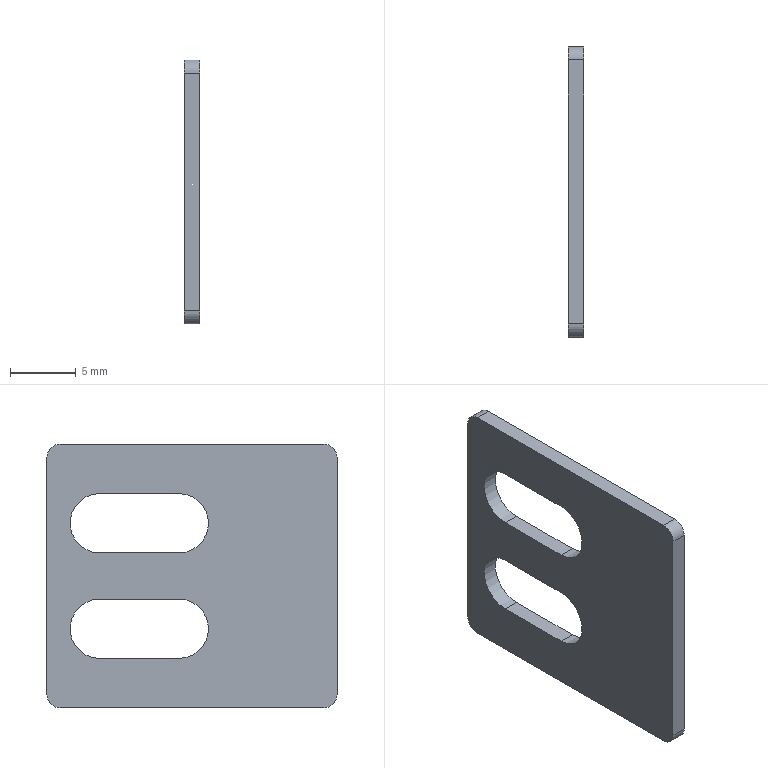Part | SolidWorks | features Fillet 1, FlatPattern 1, HoleWzd 1, SMBaseFlange 1, SheetMetal 1 | 1 solid | 18 faces | box 1.2 x 22 x 20 mm | volume 424 mm3 | plane 10 | cylinder 8 | commonest cylinder face diameters 2 x4 4.5 x4
STEP:
#1=CARTESIAN_POINT('',(-1.2,-10.,-10.));
#2=VERTEX_POINT('',#1);
#3=CARTESIAN_POINT('',(-1.2,10.,-10.));
#4=VERTEX_POINT('',#3);
#5=CARTESIAN_POINT('',(-1.2,-11.,-10.));
#6=DIRECTION('',(0.,1.,0.));
#7=VECTOR('',#6,1000.);
#8=LINE('',#5,#7);
#9=EDGE_CURVE('',#2,#4,#8,.T.);
#10=ORIENTED_EDGE('',*,*,#9,.T.);
#11=CARTESIAN_POINT('',(0.,10.,-10.));
#12=VERTEX_POINT('',#11);
#13=CARTESIAN_POINT('',(-1.2,10.,-10.));
#14=DIRECTION('',(1.,0.,0.));
#15=VECTOR('',#14,1000.);
#16=LINE('',#13,#15);
#17=EDGE_CURVE('',#4,#12,#16,.T.);
#18=ORIENTED_EDGE('',*,*,#17,.T.);
#19=CARTESIAN_POINT('',(0.,-10.,-10.));
#20=VERTEX_POINT('',#19);
#21=CARTESIAN_POINT('',(0.,-11.,-10.));
#22=DIRECTION('',(0.,1.,0.));
#23=VECTOR('',#22,1000.);
#24=LINE('',#21,#23);
#25=EDGE_CURVE('',#20,#12,#24,.T.);
#26=ORIENTED_EDGE('',*,*,#25,.F.);
#27=CARTESIAN_POINT('',(-1.2,-10.,-10.));
#28=DIRECTION('',(-1.,0.,0.));
#29=VECTOR('',#28,1000.);
#30=LINE('',#27,#29);
#31=EDGE_CURVE('',#20,#2,#30,.T.);
#32=ORIENTED_EDGE('',*,*,#31,.T.);
#33=EDGE_LOOP('',(#10,#18,#26,#32));
#34=FACE_OUTER_BOUND('',#33,.T.);
#35=CARTESIAN_POINT('',(-1.2,-11.,-10.));
#36=DIRECTION('',(0.,0.,-1.));
#37=DIRECTION('',(-1.,0.,0.));
#38=AXIS2_PLACEMENT_3D('',#35,#36,#37);
#39=PLANE('',#38);
#40=ADVANCED_FACE('',(#34),#39,.T.);
#41=CARTESIAN_POINT('',(0.,-11.,9.));
#42=VERTEX_POINT('',#41);
#43=CARTESIAN_POINT('',(0.,-11.,-9.));
#44=VERTEX_POINT('',#43);
#45=CARTESIAN_POINT('',(0.,-11.,10.));
#46=DIRECTION('',(0.,0.,-1.));
#47=VECTOR('',#46,1000.);
#48=LINE('',#45,#47);
#49=EDGE_CURVE('',#42,#44,#48,.T.);
#50=ORIENTED_EDGE('',*,*,#49,.F.);
#51=CARTESIAN_POINT('',(-1.2,-11.,9.));
#52=VERTEX_POINT('',#51);
#53=CARTESIAN_POINT('',(-1.2,-11.,9.));
#54=DIRECTION('',(-1.,0.,0.));
#55=VECTOR('',#54,1000.);
#56=LINE('',#53,#55);
#57=EDGE_CURVE('',#42,#52,#56,.T.);
#58=ORIENTED_EDGE('',*,*,#57,.T.);
#59=CARTESIAN_POINT('',(-1.2,-11.,-9.));
#60=VERTEX_POINT('',#59);
#61=CARTESIAN_POINT('',(-1.2,-11.,10.));
#62=DIRECTION('',(0.,0.,-1.));
#63=VECTOR('',#62,1000.);
#64=LINE('',#61,#63);
#65=EDGE_CURVE('',#52,#60,#64,.T.);
#66=ORIENTED_EDGE('',*,*,#65,.T.);
#67=CARTESIAN_POINT('',(-1.2,-11.,-9.));
#68=DIRECTION('',(1.,0.,0.));
#69=VECTOR('',#68,1000.);
#70=LINE('',#67,#69);
#71=EDGE_CURVE('',#60,#44,#70,.T.);
#72=ORIENTED_EDGE('',*,*,#71,.T.);
#73=EDGE_LOOP('',(#50,#58,#66,#72));
#74=FACE_OUTER_BOUND('',#73,.T.);
#75=CARTESIAN_POINT('',(-1.2,-11.,10.));
#76=DIRECTION('',(0.,-1.,0.));
#77=DIRECTION('',(0.,0.,-1.));
#78=AXIS2_PLACEMENT_3D('',#75,#76,#77);
#79=PLANE('',#78);
#80=ADVANCED_FACE('',(#74),#79,.T.);
#81=CARTESIAN_POINT('',(0.,10.,10.));
#82=VERTEX_POINT('',#81);
#83=CARTESIAN_POINT('',(0.,-10.,10.));
#84=VERTEX_POINT('',#83);
#85=CARTESIAN_POINT('',(0.,-11.,10.));
#86=DIRECTION('',(0.,-1.,0.));
#87=VECTOR('',#86,1000.);
#88=LINE('',#85,#87);
#89=EDGE_CURVE('',#82,#84,#88,.T.);
#90=ORIENTED_EDGE('',*,*,#89,.F.);
#91=CARTESIAN_POINT('',(-1.2,10.,10.));
#92=VERTEX_POINT('',#91);
#93=CARTESIAN_POINT('',(-1.2,10.,10.));
#94=DIRECTION('',(-1.,0.,0.));
#95=VECTOR('',#94,1000.);
#96=LINE('',#93,#95);
#97=EDGE_CURVE('',#82,#92,#96,.T.);
#98=ORIENTED_EDGE('',*,*,#97,.T.);
#99=CARTESIAN_POINT('',(-1.2,-10.,10.));
#100=VERTEX_POINT('',#99);
#101=CARTESIAN_POINT('',(-1.2,-11.,10.));
#102=DIRECTION('',(0.,-1.,0.));
#103=VECTOR('',#102,1000.);
#104=LINE('',#101,#103);
#105=EDGE_CURVE('',#92,#100,#104,.T.);
#106=ORIENTED_EDGE('',*,*,#105,.T.);
#107=CARTESIAN_POINT('',(-1.2,-10.,10.));
#108=DIRECTION('',(1.,0.,0.));
#109=VECTOR('',#108,1000.);
#110=LINE('',#107,#109);
#111=EDGE_CURVE('',#100,#84,#110,.T.);
#112=ORIENTED_EDGE('',*,*,#111,.T.);
#113=EDGE_LOOP('',(#90,#98,#106,#112));
#114=FACE_OUTER_BOUND('',#113,.T.);
#115=CARTESIAN_POINT('',(-1.2,-11.,10.));
#116=DIRECTION('',(0.,0.,1.));
#117=DIRECTION('',(1.,0.,0.));
#118=AXIS2_PLACEMENT_3D('',#115,#116,#117);
#119=PLANE('',#118);
#120=ADVANCED_FACE('',(#114),#119,.T.);
#121=CARTESIAN_POINT('',(-1.2,11.,-9.));
#122=VERTEX_POINT('',#121);
#123=CARTESIAN_POINT('',(-1.2,11.,9.));
#124=VERTEX_POINT('',#123);
#125=CARTESIAN_POINT('',(-1.2,11.,10.));
#126=DIRECTION('',(0.,0.,1.));
#127=VECTOR('',#126,1000.);
#128=LINE('',#125,#127);
#129=EDGE_CURVE('',#122,#124,#128,.T.);
#130=ORIENTED_EDGE('',*,*,#129,.T.);
#131=CARTESIAN_POINT('',(0.,11.,9.));
#132=VERTEX_POINT('',#131);
#133=CARTESIAN_POINT('',(-1.2,11.,9.));
#134=DIRECTION('',(1.,0.,0.));
#135=VECTOR('',#134,1000.);
#136=LINE('',#133,#135);
#137=EDGE_CURVE('',#124,#132,#136,.T.);
#138=ORIENTED_EDGE('',*,*,#137,.T.);
#139=CARTESIAN_POINT('',(0.,11.,-9.));
#140=VERTEX_POINT('',#139);
#141=CARTESIAN_POINT('',(0.,11.,10.));
#142=DIRECTION('',(0.,0.,1.));
#143=VECTOR('',#142,1000.);
#144=LINE('',#141,#143);
#145=EDGE_CURVE('',#140,#132,#144,.T.);
#146=ORIENTED_EDGE('',*,*,#145,.F.);
#147=CARTESIAN_POINT('',(-1.2,11.,-9.));
#148=DIRECTION('',(-1.,0.,0.));
#149=VECTOR('',#148,1000.);
#150=LINE('',#147,#149);
#151=EDGE_CURVE('',#140,#122,#150,.T.);
#152=ORIENTED_EDGE('',*,*,#151,.T.);
#153=EDGE_LOOP('',(#130,#138,#146,#152));
#154=FACE_OUTER_BOUND('',#153,.T.);
#155=CARTESIAN_POINT('',(-1.2,11.,10.));
#156=DIRECTION('',(0.,1.,0.));
#157=DIRECTION('',(0.,0.,1.));
#158=AXIS2_PLACEMENT_3D('',#155,#156,#157);
#159=PLANE('',#158);
#160=ADVANCED_FACE('',(#154),#159,.T.);
#161=CARTESIAN_POINT('',(-1.2,1.,-1.75));
#162=VERTEX_POINT('',#161);
#163=CARTESIAN_POINT('',(-1.2,7.,-1.75));
#164=VERTEX_POINT('',#163);
#165=CARTESIAN_POINT('',(-1.2,1.,-1.75));
#166=DIRECTION('',(0.,1.,0.));
#167=VECTOR('',#166,1000.);
#168=LINE('',#165,#167);
#169=EDGE_CURVE('',#162,#164,#168,.T.);
#170=ORIENTED_EDGE('',*,*,#169,.F.);
#171=CARTESIAN_POINT('',(-1.2,1.,-6.25));
#172=VERTEX_POINT('',#171);
#173=CARTESIAN_POINT('',(-1.2,1.,-4.));
#174=DIRECTION('',(-1.,0.,0.));
#175=DIRECTION('',(0.,0.,1.));
#176=AXIS2_PLACEMENT_3D('',#173,#174,#175);
#177=CIRCLE('',#176,2.25);
#178=EDGE_CURVE('',#172,#162,#177,.T.);
#179=ORIENTED_EDGE('',*,*,#178,.F.);
#180=CARTESIAN_POINT('',(-1.2,7.,-6.25));
#181=VERTEX_POINT('',#180);
#182=CARTESIAN_POINT('',(-1.2,1.,-6.25));
#183=DIRECTION('',(0.,1.,0.));
#184=VECTOR('',#183,1000.);
#185=LINE('',#182,#184);
#186=EDGE_CURVE('',#172,#181,#185,.T.);
#187=ORIENTED_EDGE('',*,*,#186,.T.);
#188=CARTESIAN_POINT('',(-1.2,7.,-4.));
#189=DIRECTION('',(-1.,0.,0.));
#190=DIRECTION('',(0.,0.,1.));
#191=AXIS2_PLACEMENT_3D('',#188,#189,#190);
#192=CIRCLE('',#191,2.25);
#193=EDGE_CURVE('',#164,#181,#192,.T.);
#194=ORIENTED_EDGE('',*,*,#193,.F.);
#195=EDGE_LOOP('',(#170,#179,#187,#194));
#196=FACE_BOUND('',#195,.T.);
#197=CARTESIAN_POINT('',(-1.2,1.,1.75));
#198=VERTEX_POINT('',#197);
#199=CARTESIAN_POINT('',(-1.2,1.,6.25));
#200=VERTEX_POINT('',#199);
#201=CARTESIAN_POINT('',(-1.2,1.,4.));
#202=DIRECTION('',(-1.,0.,0.));
#203=DIRECTION('',(0.,0.,1.));
#204=AXIS2_PLACEMENT_3D('',#201,#202,#203);
#205=CIRCLE('',#204,2.25);
#206=EDGE_CURVE('',#198,#200,#205,.T.);
#207=ORIENTED_EDGE('',*,*,#206,.F.);
#208=CARTESIAN_POINT('',(-1.2,7.,1.75));
#209=VERTEX_POINT('',#208);
#210=CARTESIAN_POINT('',(-1.2,1.,1.75));
#211=DIRECTION('',(0.,1.,0.));
#212=VECTOR('',#211,1000.);
#213=LINE('',#210,#212);
#214=EDGE_CURVE('',#198,#209,#213,.T.);
#215=ORIENTED_EDGE('',*,*,#214,.T.);
#216=CARTESIAN_POINT('',(-1.2,7.,6.25));
#217=VERTEX_POINT('',#216);
#218=CARTESIAN_POINT('',(-1.2,7.,4.));
#219=DIRECTION('',(-1.,0.,0.));
#220=DIRECTION('',(0.,0.,1.));
#221=AXIS2_PLACEMENT_3D('',#218,#219,#220);
#222=CIRCLE('',#221,2.25);
#223=EDGE_CURVE('',#217,#209,#222,.T.);
#224=ORIENTED_EDGE('',*,*,#223,.F.);
#225=CARTESIAN_POINT('',(-1.2,1.,6.25));
#226=DIRECTION('',(0.,1.,0.));
#227=VECTOR('',#226,1000.);
#228=LINE('',#225,#227);
#229=EDGE_CURVE('',#200,#217,#228,.T.);
#230=ORIENTED_EDGE('',*,*,#229,.F.);
#231=EDGE_LOOP('',(#207,#215,#224,#230));
#232=FACE_BOUND('',#231,.T.);
#233=ORIENTED_EDGE('',*,*,#105,.F.);
#234=CARTESIAN_POINT('',(-1.2,10.,9.));
#235=DIRECTION('',(-1.,0.,0.));
#236=DIRECTION('',(0.,0.,1.));
#237=AXIS2_PLACEMENT_3D('',#234,#235,#236);
#238=CIRCLE('',#237,1.);
#239=EDGE_CURVE('',#92,#124,#238,.T.);
#240=ORIENTED_EDGE('',*,*,#239,.T.);
#241=ORIENTED_EDGE('',*,*,#129,.F.);
#242=CARTESIAN_POINT('',(-1.2,10.,-9.));
#243=DIRECTION('',(-1.,0.,0.));
#244=DIRECTION('',(0.,0.,1.));
#245=AXIS2_PLACEMENT_3D('',#242,#243,#244);
#246=CIRCLE('',#245,1.);
#247=EDGE_CURVE('',#122,#4,#246,.T.);
#248=ORIENTED_EDGE('',*,*,#247,.T.);
#249=ORIENTED_EDGE('',*,*,#9,.F.);
#250=CARTESIAN_POINT('',(-1.2,-10.,-9.));
#251=DIRECTION('',(-1.,0.,0.));
#252=DIRECTION('',(0.,0.,1.));
#253=AXIS2_PLACEMENT_3D('',#250,#251,#252);
#254=CIRCLE('',#253,1.);
#255=EDGE_CURVE('',#2,#60,#254,.T.);
#256=ORIENTED_EDGE('',*,*,#255,.T.);
#257=ORIENTED_EDGE('',*,*,#65,.F.);
#258=CARTESIAN_POINT('',(-1.2,-10.,9.));
#259=DIRECTION('',(-1.,0.,0.));
#260=DIRECTION('',(0.,0.,1.));
#261=AXIS2_PLACEMENT_3D('',#258,#259,#260);
#262=CIRCLE('',#261,1.);
#263=EDGE_CURVE('',#52,#100,#262,.T.);
#264=ORIENTED_EDGE('',*,*,#263,.T.);
#265=EDGE_LOOP('',(#233,#240,#241,#248,#249,#256,#257,#264));
#266=FACE_OUTER_BOUND('',#265,.T.);
#267=CARTESIAN_POINT('',(-1.2,0.,0.));
#268=DIRECTION('',(-1.,0.,0.));
#269=DIRECTION('',(0.,0.,1.));
#270=AXIS2_PLACEMENT_3D('',#267,#268,#269);
#271=PLANE('',#270);
#272=ADVANCED_FACE('',(#196,#232,#266),#271,.T.);
#273=CARTESIAN_POINT('',(0.,1.,-6.25));
#274=VERTEX_POINT('',#273);
#275=CARTESIAN_POINT('',(0.,1.,-1.75));
#276=VERTEX_POINT('',#275);
#277=CARTESIAN_POINT('',(0.,1.,-4.));
#278=DIRECTION('',(-1.,0.,0.));
#279=DIRECTION('',(0.,0.,1.));
#280=AXIS2_PLACEMENT_3D('',#277,#278,#279);
#281=CIRCLE('',#280,2.25);
#282=EDGE_CURVE('',#274,#276,#281,.T.);
#283=ORIENTED_EDGE('',*,*,#282,.T.);
#284=CARTESIAN_POINT('',(0.,7.,-1.75));
#285=VERTEX_POINT('',#284);
#286=CARTESIAN_POINT('',(0.,0.,-1.75));
#287=DIRECTION('',(0.,1.,0.));
#288=VECTOR('',#287,1000.);
#289=LINE('',#286,#288);
#290=EDGE_CURVE('',#276,#285,#289,.T.);
#291=ORIENTED_EDGE('',*,*,#290,.T.);
#292=CARTESIAN_POINT('',(0.,7.,-6.25));
#293=VERTEX_POINT('',#292);
#294=CARTESIAN_POINT('',(0.,7.,-4.));
#295=DIRECTION('',(-1.,0.,0.));
#296=DIRECTION('',(0.,0.,1.));
#297=AXIS2_PLACEMENT_3D('',#294,#295,#296);
#298=CIRCLE('',#297,2.25);
#299=EDGE_CURVE('',#285,#293,#298,.T.);
#300=ORIENTED_EDGE('',*,*,#299,.T.);
#301=CARTESIAN_POINT('',(0.,0.,-6.25));
#302=DIRECTION('',(0.,-1.,0.));
#303=VECTOR('',#302,1000.);
#304=LINE('',#301,#303);
#305=EDGE_CURVE('',#293,#274,#304,.T.);
#306=ORIENTED_EDGE('',*,*,#305,.T.);
#307=EDGE_LOOP('',(#283,#291,#300,#306));
#308=FACE_BOUND('',#307,.T.);
#309=CARTESIAN_POINT('',(0.,7.,6.25));
#310=VERTEX_POINT('',#309);
#311=CARTESIAN_POINT('',(0.,7.,1.75));
#312=VERTEX_POINT('',#311);
#313=CARTESIAN_POINT('',(0.,7.,4.));
#314=DIRECTION('',(-1.,0.,0.));
#315=DIRECTION('',(0.,0.,1.));
#316=AXIS2_PLACEMENT_3D('',#313,#314,#315);
#317=CIRCLE('',#316,2.25);
#318=EDGE_CURVE('',#310,#312,#317,.T.);
#319=ORIENTED_EDGE('',*,*,#318,.T.);
#320=CARTESIAN_POINT('',(0.,1.,1.75));
#321=VERTEX_POINT('',#320);
#322=CARTESIAN_POINT('',(0.,0.,1.75));
#323=DIRECTION('',(0.,-1.,0.));
#324=VECTOR('',#323,1000.);
#325=LINE('',#322,#324);
#326=EDGE_CURVE('',#312,#321,#325,.T.);
#327=ORIENTED_EDGE('',*,*,#326,.T.);
#328=CARTESIAN_POINT('',(0.,1.,6.25));
#329=VERTEX_POINT('',#328);
#330=CARTESIAN_POINT('',(0.,1.,4.));
#331=DIRECTION('',(-1.,0.,0.));
#332=DIRECTION('',(0.,0.,1.));
#333=AXIS2_PLACEMENT_3D('',#330,#331,#332);
#334=CIRCLE('',#333,2.25);
#335=EDGE_CURVE('',#321,#329,#334,.T.);
#336=ORIENTED_EDGE('',*,*,#335,.T.);
#337=CARTESIAN_POINT('',(0.,0.,6.25));
#338=DIRECTION('',(0.,1.,0.));
#339=VECTOR('',#338,1000.);
#340=LINE('',#337,#339);
#341=EDGE_CURVE('',#329,#310,#340,.T.);
#342=ORIENTED_EDGE('',*,*,#341,.T.);
#343=EDGE_LOOP('',(#319,#327,#336,#342));
#344=FACE_BOUND('',#343,.T.);
#345=ORIENTED_EDGE('',*,*,#145,.T.);
#346=CARTESIAN_POINT('',(0.,10.,9.));
#347=DIRECTION('',(1.,0.,0.));
#348=DIRECTION('',(0.,0.,1.));
#349=AXIS2_PLACEMENT_3D('',#346,#347,#348);
#350=CIRCLE('',#349,1.);
#351=EDGE_CURVE('',#132,#82,#350,.T.);
#352=ORIENTED_EDGE('',*,*,#351,.T.);
#353=ORIENTED_EDGE('',*,*,#89,.T.);
#354=CARTESIAN_POINT('',(0.,-10.,9.));
#355=DIRECTION('',(1.,0.,0.));
#356=DIRECTION('',(0.,0.,1.));
#357=AXIS2_PLACEMENT_3D('',#354,#355,#356);
#358=CIRCLE('',#357,1.);
#359=EDGE_CURVE('',#84,#42,#358,.T.);
#360=ORIENTED_EDGE('',*,*,#359,.T.);
#361=ORIENTED_EDGE('',*,*,#49,.T.);
#362=CARTESIAN_POINT('',(0.,-10.,-9.));
#363=DIRECTION('',(1.,0.,0.));
#364=DIRECTION('',(0.,0.,1.));
#365=AXIS2_PLACEMENT_3D('',#362,#363,#364);
#366=CIRCLE('',#365,1.);
#367=EDGE_CURVE('',#44,#20,#366,.T.);
#368=ORIENTED_EDGE('',*,*,#367,.T.);
#369=ORIENTED_EDGE('',*,*,#25,.T.);
#370=CARTESIAN_POINT('',(0.,10.,-9.));
#371=DIRECTION('',(1.,0.,0.));
#372=DIRECTION('',(0.,0.,1.));
#373=AXIS2_PLACEMENT_3D('',#370,#371,#372);
#374=CIRCLE('',#373,1.);
#375=EDGE_CURVE('',#12,#140,#374,.T.);
#376=ORIENTED_EDGE('',*,*,#375,.T.);
#377=EDGE_LOOP('',(#345,#352,#353,#360,#361,#368,#369,#376));
#378=FACE_OUTER_BOUND('',#377,.T.);
#379=CARTESIAN_POINT('',(0.,0.,0.));
#380=DIRECTION('',(-1.,0.,0.));
#381=DIRECTION('',(0.,0.,1.));
#382=AXIS2_PLACEMENT_3D('',#379,#380,#381);
#383=PLANE('',#382);
#384=ADVANCED_FACE('',(#308,#344,#378),#383,.F.);
#385=CARTESIAN_POINT('',(-1.2,7.,1.75));
#386=DIRECTION('',(-1.,0.,0.));
#387=VECTOR('',#386,1000.);
#388=LINE('',#385,#387);
#389=EDGE_CURVE('',#312,#209,#388,.T.);
#390=ORIENTED_EDGE('',*,*,#389,.T.);
#391=ORIENTED_EDGE('',*,*,#214,.F.);
#392=CARTESIAN_POINT('',(-1.2,1.,1.75));
#393=DIRECTION('',(1.,0.,0.));
#394=VECTOR('',#393,1000.);
#395=LINE('',#392,#394);
#396=EDGE_CURVE('',#198,#321,#395,.T.);
#397=ORIENTED_EDGE('',*,*,#396,.T.);
#398=ORIENTED_EDGE('',*,*,#326,.F.);
#399=EDGE_LOOP('',(#390,#391,#397,#398));
#400=FACE_OUTER_BOUND('',#399,.T.);
#401=CARTESIAN_POINT('',(-1.2,1.,1.75));
#402=DIRECTION('',(0.,0.,-1.));
#403=DIRECTION('',(-1.,0.,0.));
#404=AXIS2_PLACEMENT_3D('',#401,#402,#403);
#405=PLANE('',#404);
#406=ADVANCED_FACE('',(#400),#405,.F.);
#407=CARTESIAN_POINT('',(-1.2,7.,6.25));
#408=DIRECTION('',(1.,0.,0.));
#409=VECTOR('',#408,1000.);
#410=LINE('',#407,#409);
#411=EDGE_CURVE('',#217,#310,#410,.T.);
#412=ORIENTED_EDGE('',*,*,#411,.F.);
#413=ORIENTED_EDGE('',*,*,#223,.T.);
#414=ORIENTED_EDGE('',*,*,#389,.F.);
#415=ORIENTED_EDGE('',*,*,#318,.F.);
#416=EDGE_LOOP('',(#412,#413,#414,#415));
#417=FACE_OUTER_BOUND('',#416,.T.);
#418=CARTESIAN_POINT('',(-1.2,7.,4.));
#419=DIRECTION('',(-1.,0.,0.));
#420=DIRECTION('',(0.,0.,1.));
#421=AXIS2_PLACEMENT_3D('',#418,#419,#420);
#422=CYLINDRICAL_SURFACE('',#421,2.25);
#423=ADVANCED_FACE('',(#417),#422,.F.);
#424=CARTESIAN_POINT('',(-1.2,1.,6.25));
#425=DIRECTION('',(-1.,0.,0.));
#426=VECTOR('',#425,1000.);
#427=LINE('',#424,#426);
#428=EDGE_CURVE('',#329,#200,#427,.T.);
#429=ORIENTED_EDGE('',*,*,#428,.T.);
#430=ORIENTED_EDGE('',*,*,#229,.T.);
#431=ORIENTED_EDGE('',*,*,#411,.T.);
#432=ORIENTED_EDGE('',*,*,#341,.F.);
#433=EDGE_LOOP('',(#429,#430,#431,#432));
#434=FACE_OUTER_BOUND('',#433,.T.);
#435=CARTESIAN_POINT('',(-1.2,1.,6.25));
#436=DIRECTION('',(0.,0.,1.));
#437=DIRECTION('',(1.,0.,0.));
#438=AXIS2_PLACEMENT_3D('',#435,#436,#437);
#439=PLANE('',#438);
#440=ADVANCED_FACE('',(#434),#439,.F.);
#441=ORIENTED_EDGE('',*,*,#396,.F.);
#442=ORIENTED_EDGE('',*,*,#206,.T.);
#443=ORIENTED_EDGE('',*,*,#428,.F.);
#444=ORIENTED_EDGE('',*,*,#335,.F.);
#445=EDGE_LOOP('',(#441,#442,#443,#444));
#446=FACE_OUTER_BOUND('',#445,.T.);
#447=CARTESIAN_POINT('',(-1.2,1.,4.));
#448=DIRECTION('',(-1.,0.,0.));
#449=DIRECTION('',(0.,0.,1.));
#450=AXIS2_PLACEMENT_3D('',#447,#448,#449);
#451=CYLINDRICAL_SURFACE('',#450,2.25);
#452=ADVANCED_FACE('',(#446),#451,.F.);
#453=CARTESIAN_POINT('',(-1.2,1.,-6.25));
#454=DIRECTION('',(1.,0.,0.));
#455=VECTOR('',#454,1000.);
#456=LINE('',#453,#455);
#457=EDGE_CURVE('',#172,#274,#456,.T.);
#458=ORIENTED_EDGE('',*,*,#457,.F.);
#459=ORIENTED_EDGE('',*,*,#178,.T.);
#460=CARTESIAN_POINT('',(-1.2,1.,-1.75));
#461=DIRECTION('',(-1.,0.,0.));
#462=VECTOR('',#461,1000.);
#463=LINE('',#460,#462);
#464=EDGE_CURVE('',#276,#162,#463,.T.);
#465=ORIENTED_EDGE('',*,*,#464,.F.);
#466=ORIENTED_EDGE('',*,*,#282,.F.);
#467=EDGE_LOOP('',(#458,#459,#465,#466));
#468=FACE_OUTER_BOUND('',#467,.T.);
#469=CARTESIAN_POINT('',(-1.2,1.,-4.));
#470=DIRECTION('',(-1.,0.,0.));
#471=DIRECTION('',(0.,0.,1.));
#472=AXIS2_PLACEMENT_3D('',#469,#470,#471);
#473=CYLINDRICAL_SURFACE('',#472,2.25);
#474=ADVANCED_FACE('',(#468),#473,.F.);
#475=CARTESIAN_POINT('',(-1.2,7.,-1.75));
#476=DIRECTION('',(1.,0.,0.));
#477=VECTOR('',#476,1000.);
#478=LINE('',#475,#477);
#479=EDGE_CURVE('',#164,#285,#478,.T.);
#480=ORIENTED_EDGE('',*,*,#479,.F.);
#481=ORIENTED_EDGE('',*,*,#193,.T.);
#482=CARTESIAN_POINT('',(-1.2,7.,-6.25));
#483=DIRECTION('',(-1.,0.,0.));
#484=VECTOR('',#483,1000.);
#485=LINE('',#482,#484);
#486=EDGE_CURVE('',#293,#181,#485,.T.);
#487=ORIENTED_EDGE('',*,*,#486,.F.);
#488=ORIENTED_EDGE('',*,*,#299,.F.);
#489=EDGE_LOOP('',(#480,#481,#487,#488));
#490=FACE_OUTER_BOUND('',#489,.T.);
#491=CARTESIAN_POINT('',(-1.2,7.,-4.));
#492=DIRECTION('',(-1.,0.,0.));
#493=DIRECTION('',(0.,0.,1.));
#494=AXIS2_PLACEMENT_3D('',#491,#492,#493);
#495=CYLINDRICAL_SURFACE('',#494,2.25);
#496=ADVANCED_FACE('',(#490),#495,.F.);
#497=ORIENTED_EDGE('',*,*,#464,.T.);
#498=ORIENTED_EDGE('',*,*,#169,.T.);
#499=ORIENTED_EDGE('',*,*,#479,.T.);
#500=ORIENTED_EDGE('',*,*,#290,.F.);
#501=EDGE_LOOP('',(#497,#498,#499,#500));
#502=FACE_OUTER_BOUND('',#501,.T.);
#503=CARTESIAN_POINT('',(-1.2,1.,-1.75));
#504=DIRECTION('',(0.,0.,1.));
#505=DIRECTION('',(1.,0.,0.));
#506=AXIS2_PLACEMENT_3D('',#503,#504,#505);
#507=PLANE('',#506);
#508=ADVANCED_FACE('',(#502),#507,.F.);
#509=ORIENTED_EDGE('',*,*,#486,.T.);
#510=ORIENTED_EDGE('',*,*,#186,.F.);
#511=ORIENTED_EDGE('',*,*,#457,.T.);
#512=ORIENTED_EDGE('',*,*,#305,.F.);
#513=EDGE_LOOP('',(#509,#510,#511,#512));
#514=FACE_OUTER_BOUND('',#513,.T.);
#515=CARTESIAN_POINT('',(-1.2,1.,-6.25));
#516=DIRECTION('',(0.,0.,-1.));
#517=DIRECTION('',(-1.,0.,0.));
#518=AXIS2_PLACEMENT_3D('',#515,#516,#517);
#519=PLANE('',#518);
#520=ADVANCED_FACE('',(#514),#519,.F.);
#521=ORIENTED_EDGE('',*,*,#239,.F.);
#522=ORIENTED_EDGE('',*,*,#97,.F.);
#523=ORIENTED_EDGE('',*,*,#351,.F.);
#524=ORIENTED_EDGE('',*,*,#137,.F.);
#525=EDGE_LOOP('',(#521,#522,#523,#524));
#526=FACE_OUTER_BOUND('',#525,.T.);
#527=CARTESIAN_POINT('',(-1.2,10.,9.));
#528=DIRECTION('',(1.,0.,0.));
#529=DIRECTION('',(0.,0.,-1.));
#530=AXIS2_PLACEMENT_3D('',#527,#528,#529);
#531=CYLINDRICAL_SURFACE('',#530,1.);
#532=ADVANCED_FACE('',(#526),#531,.T.);
#533=ORIENTED_EDGE('',*,*,#263,.F.);
#534=ORIENTED_EDGE('',*,*,#57,.F.);
#535=ORIENTED_EDGE('',*,*,#359,.F.);
#536=ORIENTED_EDGE('',*,*,#111,.F.);
#537=EDGE_LOOP('',(#533,#534,#535,#536));
#538=FACE_OUTER_BOUND('',#537,.T.);
#539=CARTESIAN_POINT('',(-1.2,-10.,9.));
#540=DIRECTION('',(1.,0.,0.));
#541=DIRECTION('',(0.,0.,-1.));
#542=AXIS2_PLACEMENT_3D('',#539,#540,#541);
#543=CYLINDRICAL_SURFACE('',#542,1.);
#544=ADVANCED_FACE('',(#538),#543,.T.);
#545=ORIENTED_EDGE('',*,*,#247,.F.);
#546=ORIENTED_EDGE('',*,*,#151,.F.);
#547=ORIENTED_EDGE('',*,*,#375,.F.);
#548=ORIENTED_EDGE('',*,*,#17,.F.);
#549=EDGE_LOOP('',(#545,#546,#547,#548));
#550=FACE_OUTER_BOUND('',#549,.T.);
#551=CARTESIAN_POINT('',(-1.2,10.,-9.));
#552=DIRECTION('',(1.,0.,0.));
#553=DIRECTION('',(0.,0.,-1.));
#554=AXIS2_PLACEMENT_3D('',#551,#552,#553);
#555=CYLINDRICAL_SURFACE('',#554,1.);
#556=ADVANCED_FACE('',(#550),#555,.T.);
#557=ORIENTED_EDGE('',*,*,#255,.F.);
#558=ORIENTED_EDGE('',*,*,#31,.F.);
#559=ORIENTED_EDGE('',*,*,#367,.F.);
#560=ORIENTED_EDGE('',*,*,#71,.F.);
#561=EDGE_LOOP('',(#557,#558,#559,#560));
#562=FACE_OUTER_BOUND('',#561,.T.);
#563=CARTESIAN_POINT('',(-1.2,-10.,-9.));
#564=DIRECTION('',(1.,0.,0.));
#565=DIRECTION('',(0.,0.,-1.));
#566=AXIS2_PLACEMENT_3D('',#563,#564,#565);
#567=CYLINDRICAL_SURFACE('',#566,1.);
#568=ADVANCED_FACE('',(#562),#567,.T.);
#569=CLOSED_SHELL('',(#40,#80,#120,#160,#272,#384,#406,#423,#440,#452,#474,#496,#508,#520,#532,#544,#556,#568));
#570=MANIFOLD_SOLID_BREP('',#569);
#571=CARTESIAN_POINT('',(0.,0.,0.));
#572=DIRECTION('',(0.,0.,1.));
#573=DIRECTION('',(1.,0.,0.));
#574=AXIS2_PLACEMENT_3D('',#571,#572,#573);
#575=(LENGTH_UNIT()NAMED_UNIT(*)SI_UNIT(.MILLI.,.METRE.));
#576=UNCERTAINTY_MEASURE_WITH_UNIT(LENGTH_MEASURE(0.00001),#575,'','');
#577=(NAMED_UNIT(*)PLANE_ANGLE_UNIT()SI_UNIT($,.RADIAN.));
#578=(NAMED_UNIT(*)SI_UNIT($,.STERADIAN.)SOLID_ANGLE_UNIT());
#579=(GEOMETRIC_REPRESENTATION_CONTEXT(3)GLOBAL_UNCERTAINTY_ASSIGNED_CONTEXT((#576))GLOBAL_UNIT_ASSIGNED_CONTEXT((#575,#577,#578))REPRESENTATION_CONTEXT('',''));
#580=ADVANCED_BREP_SHAPE_REPRESENTATION('',(#570,#574),#579);